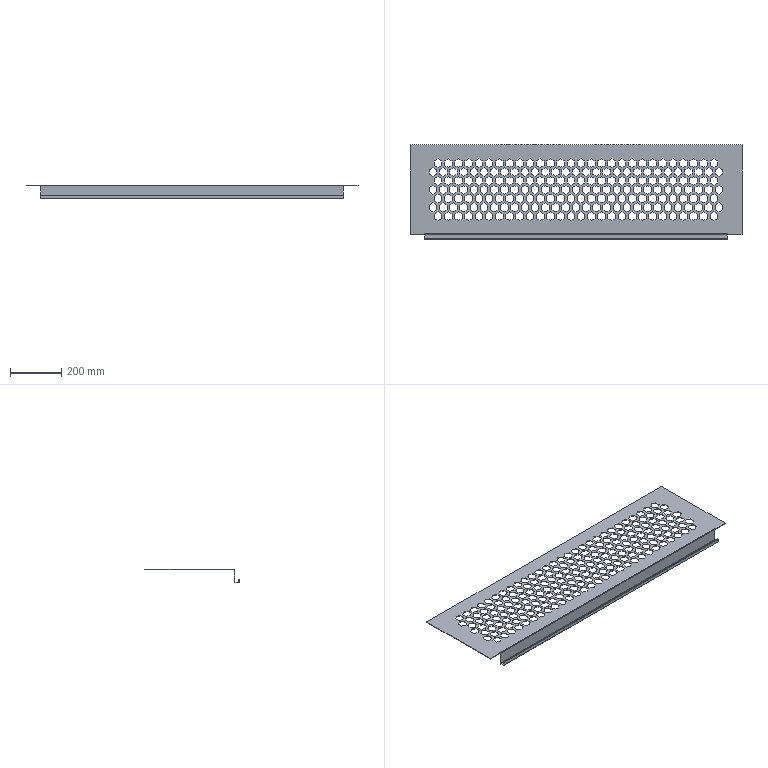Part | SolidWorks | features BaseBody 1 | 1 solid | 1232 faces | box 1300 x 370 x 54 mm | volume 795741 mm3 | plane 1226 | cylinder 6 | commonest cylinder face diameters 2 x3 6 x3